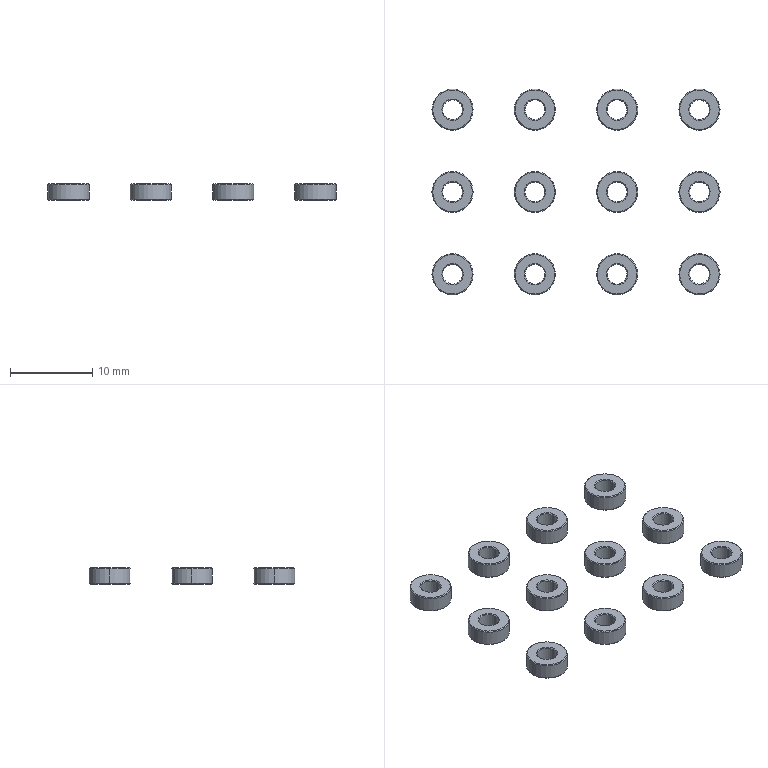NC program | NX | posted with a generic post | part box 35 x 25 x 2 mm
Lines 48 to 911 of 5177:
(ZLEVEL_PROFILE , TOOL : D4)
N88 T04 M6
N90 G54
N92 G17 G0 G90 X0.328 Y-1.531 S9500 M3
N94 G43 Z30. H4
N96 Z1.5
N98 G94 G1 X-0.348 Y-1.151 Z1.459 F1000.
N100 X-1.299 Y-0.146 Z1.387
N102 X-1.799 Y0.78 Z1.332
N104 X-2.099 Y1.969 Z1.267
N106 X-2.1 Y2.5 Z1.24
N108 Y3.026 Z1.212
N110 X-1.743 Y4.354 Z1.14
N112 X-1.012 Y5.517 Z1.068
N114 X0.029 Y6.415 Z0.996
N116 X1.287 Y6.968 Z0.924
N118 X2.653 Y7.127 Z0.852
N120 X4.005 Y6.879 Z0.78
N122 X4.954 Y6.426 Z0.725
N124 X6.004 Y5.526 Z0.652
N126 X6.742 Y4.356 Z0.58
N128 X7.101 Y3.021 Z0.507
N130 X7.099 Y1.969 Z0.452
N132 X6.909 Y1.087 Z0.405
N134 X6.551 Y0.258 Z0.358
N136 X5.94 Y-0.599 Z0.302
N138 X4.871 Y-1.477 Z0.23
N140 X3.59 Y-2. Z0.157
N142 X2.211 Y-2.121 Z0.085
N144 X0.858 Y-1.829 Z0.012
N146 X-0.348 Y-1.151 Z-0.06
N148 X-1.299 Y-0.146 Z-0.133
N150 X-1.799 Y0.78 Z-0.188
N152 X-2.099 Y1.969 Z-0.252
N154 X-2.1 Y2.5 Z-0.28
N156 G2 X2.5 Y7.1 R4.6 F2500.
N158 X-2.1 Y2.5 R-4.6
N160 G1 X-2.094 Y2.743 Z-0.284
N162 X-2.074 Y2.985 Z-0.288
N164 X-2.042 Y3.226 Z-0.293
N166 X-1.998 Y3.465 Z-0.297
N168 X-1.94 Y3.701 Z-0.301
N170 X-1.871 Y3.934 Z-0.305
N172 X-1.789 Y4.163 Z-0.31
N174 X-1.695 Y4.387 Z-0.314
N176 X-1.59 Y4.606 Z-0.318
N178 X-1.473 Y4.819 Z-0.322
N180 X-1.345 Y5.026 Z-0.327
N182 X-1.206 Y5.225 Z-0.331
N184 X-1.057 Y5.417 Z-0.335
N186 X-0.898 Y5.601 Z-0.339
N188 X-0.729 Y5.776 Z-0.344
N190 X-0.552 Y5.942 Z-0.348
N192 X-0.366 Y6.098 Z-0.352
N194 X-0.172 Y6.245 Z-0.356
N196 X0.03 Y6.38 Z-0.361
N198 X0.238 Y6.505 Z-0.365
N200 X0.453 Y6.619 Z-0.369
N202 X0.673 Y6.722 Z-0.373
N204 X0.899 Y6.812 Z-0.378
N206 X1.129 Y6.891 Z-0.382
N208 X1.362 Y6.957 Z-0.386
N210 X1.599 Y7.011 Z-0.39
N212 X1.839 Y7.052 Z-0.395
N214 X2.08 Y7.081 Z-0.399
N216 X2.323 Y7.097 Z-0.403
N218 X2.566 Y7.1 Z-0.407
N220 X2.809 Y7.09 Z-0.412
N222 X3.051 Y7.067 Z-0.416
N224 X3.291 Y7.031 Z-0.42
N226 X3.529 Y6.983 Z-0.424
N228 X3.765 Y6.923 Z-0.428
N230 X3.996 Y6.85 Z-0.433
N232 X4.224 Y6.765 Z-0.437
N234 X4.447 Y6.668 Z-0.441
N236 X4.664 Y6.559 Z-0.445
N238 X4.876 Y6.439 Z-0.45
N240 X5.08 Y6.308 Z-0.454
N242 X5.278 Y6.167 Z-0.458
N244 X5.468 Y6.015 Z-0.462
N246 X5.649 Y5.853 Z-0.467
N248 X5.822 Y5.682 Z-0.471
N250 X5.985 Y5.502 Z-0.475
N252 X6.139 Y5.314 Z-0.479
N254 X6.282 Y5.118 Z-0.484
N256 X6.415 Y4.915 Z-0.488
N258 X6.537 Y4.704 Z-0.492
N260 X6.648 Y4.488 Z-0.496
N262 X6.747 Y4.266 Z-0.501
N264 X6.835 Y4.039 Z-0.505
N266 X6.91 Y3.808 Z-0.509
N268 X6.973 Y3.574 Z-0.513
N270 X7.023 Y3.336 Z-0.518
N272 X7.061 Y3.096 Z-0.522
N274 X7.086 Y2.854 Z-0.526
N276 X7.099 Y2.611 Z-0.53
N278 X7.098 Y2.368 Z-0.535
N280 X7.085 Y2.126 Z-0.539
N282 X7.059 Y1.884 Z-0.543
N284 X7.02 Y1.644 Z-0.547
N286 X6.968 Y1.407 Z-0.552
N288 X6.904 Y1.172 Z-0.556
N290 X6.828 Y0.942 Z-0.56
N292 G2 X-2.1 Y2.5 R4.6
N294 G1 X-2.094 Y2.743 Z-0.564
N296 X-2.074 Y2.985 Z-0.568
N298 X-2.042 Y3.226 Z-0.573
N300 X-1.998 Y3.465 Z-0.577
N302 X-1.94 Y3.701 Z-0.581
N304 X-1.871 Y3.934 Z-0.585
N306 X-1.789 Y4.163 Z-0.59
N308 X-1.695 Y4.387 Z-0.594
N310 X-1.59 Y4.606 Z-0.598
N312 X-1.473 Y4.819 Z-0.602
N314 X-1.345 Y5.026 Z-0.607
N316 X-1.206 Y5.225 Z-0.611
N318 X-1.057 Y5.417 Z-0.615
N320 X-0.898 Y5.601 Z-0.619
N322 X-0.729 Y5.776 Z-0.624
N324 X-0.552 Y5.942 Z-0.628
N326 X-0.366 Y6.098 Z-0.632
N328 X-0.172 Y6.245 Z-0.636
N330 X0.03 Y6.38 Z-0.641
N332 X0.238 Y6.505 Z-0.645
N334 X0.453 Y6.619 Z-0.649
N336 X0.673 Y6.722 Z-0.653
N338 X0.899 Y6.812 Z-0.658
N340 X1.129 Y6.891 Z-0.662
N342 X1.362 Y6.957 Z-0.666
N344 X1.599 Y7.011 Z-0.67
N346 X1.839 Y7.052 Z-0.675
N348 X2.08 Y7.081 Z-0.679
N350 X2.323 Y7.097 Z-0.683
N352 X2.566 Y7.1 Z-0.687
N354 X2.809 Y7.09 Z-0.692
N356 X3.051 Y7.067 Z-0.696
N358 X3.291 Y7.031 Z-0.7
N360 X3.529 Y6.983 Z-0.704
N362 X3.765 Y6.923 Z-0.708
N364 X3.996 Y6.85 Z-0.713
N366 X4.224 Y6.765 Z-0.717
N368 X4.447 Y6.668 Z-0.721
N370 X4.664 Y6.559 Z-0.725
N372 X4.876 Y6.439 Z-0.73
N374 X5.08 Y6.308 Z-0.734
N376 X5.278 Y6.167 Z-0.738
N378 X5.468 Y6.015 Z-0.742
N380 X5.649 Y5.853 Z-0.747
N382 X5.822 Y5.682 Z-0.751
N384 X5.985 Y5.502 Z-0.755
N386 X6.139 Y5.314 Z-0.759
N388 X6.282 Y5.118 Z-0.764
N390 X6.415 Y4.915 Z-0.768
N392 X6.537 Y4.704 Z-0.772
N394 X6.648 Y4.488 Z-0.776
N396 X6.747 Y4.266 Z-0.781
N398 X6.835 Y4.039 Z-0.785
N400 X6.91 Y3.808 Z-0.789
N402 X6.973 Y3.574 Z-0.793
N404 X7.023 Y3.336 Z-0.798
N406 X7.061 Y3.096 Z-0.802
N408 X7.086 Y2.854 Z-0.806
N410 X7.099 Y2.611 Z-0.81
N412 X7.098 Y2.368 Z-0.815
N414 X7.085 Y2.126 Z-0.819
N416 X7.059 Y1.884 Z-0.823
N418 X7.02 Y1.644 Z-0.827
N420 X6.968 Y1.407 Z-0.832
N422 X6.904 Y1.172 Z-0.836
N424 X6.828 Y0.942 Z-0.84
N426 G2 X-2.1 Y2.5 R4.6
N428 G1 X-2.094 Y2.743 Z-0.844
N430 X-2.074 Y2.985 Z-0.848
N432 X-2.042 Y3.226 Z-0.853
N434 X-1.998 Y3.465 Z-0.857
N436 X-1.94 Y3.701 Z-0.861
N438 X-1.871 Y3.934 Z-0.865
N440 X-1.789 Y4.163 Z-0.87
N442 X-1.695 Y4.387 Z-0.874
N444 X-1.59 Y4.606 Z-0.878
N446 X-1.473 Y4.819 Z-0.882
N448 X-1.345 Y5.026 Z-0.887
N450 X-1.206 Y5.225 Z-0.891
N452 X-1.057 Y5.417 Z-0.895
N454 X-0.898 Y5.601 Z-0.899
N456 X-0.729 Y5.776 Z-0.904
N458 X-0.552 Y5.942 Z-0.908
N460 X-0.366 Y6.098 Z-0.912
N462 X-0.172 Y6.245 Z-0.916
N464 X0.03 Y6.38 Z-0.921
N466 X0.238 Y6.505 Z-0.925
N468 X0.453 Y6.619 Z-0.929
N470 X0.673 Y6.722 Z-0.933
N472 X0.899 Y6.812 Z-0.938
N474 X1.129 Y6.891 Z-0.942
N476 X1.362 Y6.957 Z-0.946
N478 X1.599 Y7.011 Z-0.95
N480 X1.839 Y7.052 Z-0.955
N482 X2.08 Y7.081 Z-0.959
N484 X2.323 Y7.097 Z-0.963
N486 X2.566 Y7.1 Z-0.967
N488 X2.809 Y7.09 Z-0.972
N490 X3.051 Y7.067 Z-0.976
N492 X3.291 Y7.031 Z-0.98
N494 X3.529 Y6.983 Z-0.984
N496 X3.765 Y6.923 Z-0.988
N498 X3.996 Y6.85 Z-0.993
N500 X4.224 Y6.765 Z-0.997
N502 X4.447 Y6.668 Z-1.001
N504 X4.664 Y6.559 Z-1.005
N506 X4.876 Y6.439 Z-1.01
N508 X5.08 Y6.308 Z-1.014
N510 X5.278 Y6.167 Z-1.018
N512 X5.468 Y6.015 Z-1.022
N514 X5.649 Y5.853 Z-1.027
N516 X5.822 Y5.682 Z-1.031
N518 X5.985 Y5.502 Z-1.035
N520 X6.139 Y5.314 Z-1.039
N522 X6.282 Y5.118 Z-1.044
N524 X6.415 Y4.915 Z-1.048
N526 X6.537 Y4.704 Z-1.052
N528 X6.648 Y4.488 Z-1.056
N530 X6.747 Y4.266 Z-1.061
N532 X6.835 Y4.039 Z-1.065
N534 X6.91 Y3.808 Z-1.069
N536 X6.973 Y3.574 Z-1.073
N538 X7.023 Y3.336 Z-1.078
N540 X7.061 Y3.096 Z-1.082
N542 X7.086 Y2.854 Z-1.086
N544 X7.099 Y2.611 Z-1.09
N546 X7.098 Y2.368 Z-1.095
N548 X7.085 Y2.126 Z-1.099
N550 X7.059 Y1.884 Z-1.103
N552 X7.02 Y1.644 Z-1.107
N554 X6.968 Y1.407 Z-1.112
N556 X6.904 Y1.172 Z-1.116
N558 X6.828 Y0.942 Z-1.12
N560 G2 X-2.1 Y2.5 R4.6
N562 G1 X-2.094 Y2.743 Z-1.124
N564 X-2.074 Y2.985 Z-1.128
N566 X-2.042 Y3.226 Z-1.133
N568 X-1.998 Y3.465 Z-1.137
N570 X-1.94 Y3.701 Z-1.141
N572 X-1.871 Y3.934 Z-1.145
N574 X-1.789 Y4.163 Z-1.15
N576 X-1.695 Y4.387 Z-1.154
N578 X-1.59 Y4.606 Z-1.158
N580 X-1.473 Y4.819 Z-1.162
N582 X-1.345 Y5.026 Z-1.167
N584 X-1.206 Y5.225 Z-1.171
N586 X-1.057 Y5.417 Z-1.175
N588 X-0.898 Y5.601 Z-1.179
N590 X-0.729 Y5.776 Z-1.184
N592 X-0.552 Y5.942 Z-1.188
N594 X-0.366 Y6.098 Z-1.192
N596 X-0.172 Y6.245 Z-1.196
N598 X0.03 Y6.38 Z-1.201
N600 X0.238 Y6.505 Z-1.205
N602 X0.453 Y6.619 Z-1.209
N604 X0.673 Y6.722 Z-1.213
N606 X0.899 Y6.812 Z-1.218
N608 X1.129 Y6.891 Z-1.222
N610 X1.362 Y6.957 Z-1.226
N612 X1.599 Y7.011 Z-1.23
N614 X1.839 Y7.052 Z-1.235
N616 X2.08 Y7.081 Z-1.239
N618 X2.323 Y7.097 Z-1.243
N620 X2.566 Y7.1 Z-1.247
N622 X2.809 Y7.09 Z-1.252
N624 X3.051 Y7.067 Z-1.256
N626 X3.291 Y7.031 Z-1.26
N628 X3.529 Y6.983 Z-1.264
N630 X3.765 Y6.923 Z-1.268
N632 X3.996 Y6.85 Z-1.273
N634 X4.224 Y6.765 Z-1.277
N636 X4.447 Y6.668 Z-1.281
N638 X4.664 Y6.559 Z-1.285
N640 X4.876 Y6.439 Z-1.29
N642 X5.08 Y6.308 Z-1.294
N644 X5.278 Y6.167 Z-1.298
N646 X5.468 Y6.015 Z-1.302
N648 X5.649 Y5.853 Z-1.307
N650 X5.822 Y5.682 Z-1.311
N652 X5.985 Y5.502 Z-1.315
N654 X6.139 Y5.314 Z-1.319
N656 X6.282 Y5.118 Z-1.324
N658 X6.415 Y4.915 Z-1.328
N660 X6.537 Y4.704 Z-1.332
N662 X6.648 Y4.488 Z-1.336
N664 X6.747 Y4.266 Z-1.341
N666 X6.835 Y4.039 Z-1.345
N668 X6.91 Y3.808 Z-1.349
N670 X6.973 Y3.574 Z-1.353
N672 X7.023 Y3.336 Z-1.358
N674 X7.061 Y3.096 Z-1.362
N676 X7.086 Y2.854 Z-1.366
N678 X7.099 Y2.611 Z-1.37
N680 X7.098 Y2.368 Z-1.375
N682 X7.085 Y2.126 Z-1.379
N684 X7.059 Y1.884 Z-1.383
N686 X7.02 Y1.644 Z-1.387
N688 X6.968 Y1.407 Z-1.392
N690 X6.904 Y1.172 Z-1.396
N692 X6.828 Y0.942 Z-1.4
N694 G2 X0.942 Y-1.828 R4.6
N696 X6.828 Y0.942 R-4.6
N698 G1 Z0.1
N700 G0 Z53.
N702 X16.567 Y0.295
N704 Z1.5
N706 G1 X16.551 Y0.258 Z1.498 F1000.
N708 X15.94 Y-0.599 Z1.443
N710 X15.1 Y-1.331 Z1.384
N712 X14.11 Y-1.841 Z1.326
N714 X13.026 Y-2.1 Z1.268
N716 X11.974 Z1.212
N718 X10.711 Y-1.77 Z1.144
N720 X9.59 Y-1.101 Z1.076
N722 X8.701 Y-0.146 Z1.007
N724 X8.201 Y0.78 Z0.952
N726 X7.901 Y1.969 Z0.888
N728 X7.899 Y3.021 Z0.833
N730 X8.256 Y4.35 Z0.761
N732 X8.986 Y5.515 Z0.689
N734 X10.027 Y6.414 Z0.616
N736 X11.286 Y6.968 Z0.544
N738 X12.652 Y7.128 Z0.472
N740 X14.005 Y6.879 Z0.4
N742 X14.954 Y6.426 Z0.345
N744 X16.004 Y5.526 Z0.273
N746 X16.742 Y4.356 Z0.2
N748 X17.101 Y3.021 Z0.128
N750 X17.099 Y1.969 Z0.072
N752 X16.909 Y1.087 Z0.025
N754 X16.551 Y0.258 Z-0.022
N756 X15.94 Y-0.599 Z-0.077
N758 X15.1 Y-1.331 Z-0.136
N760 X14.11 Y-1.841 Z-0.194
N762 X13.026 Y-2.1 Z-0.252
N764 X12.5 Z-0.28
N766 G2 X7.9 Y2.5 R4.6 F2500.
N768 X12.5 Y-2.1 R-4.6
N770 G1 X12.257 Y-2.094 Z-0.284
N772 X12.015 Y-2.074 Z-0.288
N774 X11.774 Y-2.042 Z-0.293
N776 X11.535 Y-1.998 Z-0.297
N778 X11.299 Y-1.94 Z-0.301
N780 X11.066 Y-1.871 Z-0.305
N782 X10.837 Y-1.789 Z-0.31
N784 X10.613 Y-1.695 Z-0.314
N786 X10.394 Y-1.59 Z-0.318
N788 X10.181 Y-1.473 Z-0.322
N790 X9.974 Y-1.345 Z-0.327
N792 X9.775 Y-1.206 Z-0.331
N794 X9.583 Y-1.057 Z-0.335
N796 X9.399 Y-0.898 Z-0.339
N798 X9.224 Y-0.729 Z-0.344
N800 X9.058 Y-0.552 Z-0.348
N802 X8.902 Y-0.366 Z-0.352
N804 X8.755 Y-0.172 Z-0.356
N806 X8.62 Y0.03 Z-0.361
N808 X8.495 Y0.238 Z-0.365
N810 X8.381 Y0.453 Z-0.369
N812 X8.278 Y0.673 Z-0.373
N814 X8.188 Y0.899 Z-0.378
N816 X8.109 Y1.129 Z-0.382
N818 X8.043 Y1.362 Z-0.386
N820 X7.989 Y1.599 Z-0.39
N822 X7.948 Y1.839 Z-0.395
N824 X7.919 Y2.08 Z-0.399
N826 X7.903 Y2.323 Z-0.403
N828 X7.9 Y2.566 Z-0.407
N830 X7.91 Y2.809 Z-0.412
N832 X7.933 Y3.051 Z-0.416
N834 X7.969 Y3.291 Z-0.42
N836 X8.017 Y3.529 Z-0.424
N838 X8.077 Y3.765 Z-0.428
N840 X8.15 Y3.996 Z-0.433
N842 X8.235 Y4.224 Z-0.437
N844 X8.332 Y4.447 Z-0.441
N846 X8.441 Y4.664 Z-0.445
N848 X8.561 Y4.876 Z-0.45
N850 X8.692 Y5.08 Z-0.454
N852 X8.833 Y5.278 Z-0.458
N854 X8.985 Y5.468 Z-0.462
N856 X9.147 Y5.649 Z-0.467
N858 X9.318 Y5.822 Z-0.471
N860 X9.498 Y5.985 Z-0.475
N862 X9.686 Y6.139 Z-0.479
N864 X9.882 Y6.282 Z-0.484
N866 X10.085 Y6.415 Z-0.488
N868 X10.296 Y6.537 Z-0.492
N870 X10.512 Y6.648 Z-0.496
N872 X10.734 Y6.747 Z-0.501
N874 X10.961 Y6.835 Z-0.505
N876 X11.192 Y6.91 Z-0.509
N878 X11.426 Y6.973 Z-0.513
N880 X11.664 Y7.023 Z-0.518
N882 X11.904 Y7.061 Z-0.522
N884 X12.146 Y7.086 Z-0.526
N886 X12.389 Y7.099 Z-0.53
N888 X12.632 Y7.098 Z-0.535
N890 X12.874 Y7.085 Z-0.539
N892 X13.116 Y7.059 Z-0.543
N894 X13.356 Y7.02 Z-0.547
N896 X13.593 Y6.968 Z-0.552
N898 X13.828 Y6.904 Z-0.556
N900 X14.058 Y6.828 Z-0.56
N902 G2 X12.5 Y-2.1 R4.6
N904 G1 X12.257 Y-2.094 Z-0.564
N906 X12.015 Y-2.074 Z-0.568
N908 X11.774 Y-2.042 Z-0.573
N910 X11.535 Y-1.998 Z-0.577
N912 X11.299 Y-1.94 Z-0.581
N914 X11.066 Y-1.871 Z-0.585
N916 X10.837 Y-1.789 Z-0.59
N918 X10.613 Y-1.695 Z-0.594
N920 X10.394 Y-1.59 Z-0.598
N922 X10.181 Y-1.473 Z-0.602
N924 X9.974 Y-1.345 Z-0.607
N926 X9.775 Y-1.206 Z-0.611
N928 X9.583 Y-1.057 Z-0.615
N930 X9.399 Y-0.898 Z-0.619
N932 X9.224 Y-0.729 Z-0.624
N934 X9.058 Y-0.552 Z-0.628
N936 X8.902 Y-0.366 Z-0.632
N938 X8.755 Y-0.172 Z-0.636
N940 X8.62 Y0.03 Z-0.641
N942 X8.495 Y0.238 Z-0.645
N944 X8.381 Y0.453 Z-0.649
N946 X8.278 Y0.673 Z-0.653
N948 X8.188 Y0.899 Z-0.658
N950 X8.109 Y1.129 Z-0.662
N952 X8.043 Y1.362 Z-0.666
N954 X7.989 Y1.599 Z-0.67
N956 X7.948 Y1.839 Z-0.675
N958 X7.919 Y2.08 Z-0.679
N960 X7.903 Y2.323 Z-0.683
N962 X7.9 Y2.566 Z-0.687
N964 X7.91 Y2.809 Z-0.692
N966 X7.933 Y3.051 Z-0.696
N968 X7.969 Y3.291 Z-0.7
N970 X8.017 Y3.529 Z-0.704
N972 X8.077 Y3.765 Z-0.708
N974 X8.15 Y3.996 Z-0.713
N976 X8.235 Y4.224 Z-0.717
N978 X8.332 Y4.447 Z-0.721
N980 X8.441 Y4.664 Z-0.725
N982 X8.561 Y4.876 Z-0.73
N984 X8.692 Y5.08 Z-0.734
N986 X8.833 Y5.278 Z-0.738
N988 X8.985 Y5.468 Z-0.742
N990 X9.147 Y5.649 Z-0.747
N992 X9.318 Y5.822 Z-0.751
N994 X9.498 Y5.985 Z-0.755
N996 X9.686 Y6.139 Z-0.759
N998 X9.882 Y6.282 Z-0.764
N1000 X10.085 Y6.415 Z-0.768
N1002 X10.296 Y6.537 Z-0.772
N1004 X10.512 Y6.648 Z-0.776
N1006 X10.734 Y6.747 Z-0.781
N1008 X10.961 Y6.835 Z-0.785
N1010 X11.192 Y6.91 Z-0.789
N1012 X11.426 Y6.973 Z-0.793
N1014 X11.664 Y7.023 Z-0.798
N1016 X11.904 Y7.061 Z-0.802
N1018 X12.146 Y7.086 Z-0.806
N1020 X12.389 Y7.099 Z-0.81
N1022 X12.632 Y7.098 Z-0.815
N1024 X12.874 Y7.085 Z-0.819
N1026 X13.116 Y7.059 Z-0.823
N1028 X13.356 Y7.02 Z-0.827
N1030 X13.593 Y6.968 Z-0.832
N1032 X13.828 Y6.904 Z-0.836
N1034 X14.058 Y6.828 Z-0.84
N1036 G2 X12.5 Y-2.1 R4.6
N1038 G1 X12.257 Y-2.094 Z-0.844
N1040 X12.015 Y-2.074 Z-0.848
N1042 X11.774 Y-2.042 Z-0.853
N1044 X11.535 Y-1.998 Z-0.857
N1046 X11.299 Y-1.94 Z-0.861
N1048 X11.066 Y-1.871 Z-0.865
N1050 X10.837 Y-1.789 Z-0.87
N1052 X10.613 Y-1.695 Z-0.874
N1054 X10.394 Y-1.59 Z-0.878
N1056 X10.181 Y-1.473 Z-0.882
N1058 X9.974 Y-1.345 Z-0.887
N1060 X9.775 Y-1.206 Z-0.891
N1062 X9.583 Y-1.057 Z-0.895
N1064 X9.399 Y-0.898 Z-0.899
N1066 X9.224 Y-0.729 Z-0.904
N1068 X9.058 Y-0.552 Z-0.908
N1070 X8.902 Y-0.366 Z-0.912
N1072 X8.755 Y-0.172 Z-0.916
N1074 X8.62 Y0.03 Z-0.921
N1076 X8.495 Y0.238 Z-0.925
N1078 X8.381 Y0.453 Z-0.929
N1080 X8.278 Y0.673 Z-0.933
N1082 X8.188 Y0.899 Z-0.938
N1084 X8.109 Y1.129 Z-0.942
N1086 X8.043 Y1.362 Z-0.946
N1088 X7.989 Y1.599 Z-0.95
N1090 X7.948 Y1.839 Z-0.955
N1092 X7.919 Y2.08 Z-0.959
N1094 X7.903 Y2.323 Z-0.963
N1096 X7.9 Y2.566 Z-0.967
N1098 X7.91 Y2.809 Z-0.972
N1100 X7.933 Y3.051 Z-0.976
N1102 X7.969 Y3.291 Z-0.98
N1104 X8.017 Y3.529 Z-0.984
N1106 X8.077 Y3.765 Z-0.988
N1108 X8.15 Y3.996 Z-0.993
N1110 X8.235 Y4.224 Z-0.997
N1112 X8.332 Y4.447 Z-1.001
N1114 X8.441 Y4.664 Z-1.005
N1116 X8.561 Y4.876 Z-1.01
N1118 X8.692 Y5.08 Z-1.014
N1120 X8.833 Y5.278 Z-1.018
N1122 X8.985 Y5.468 Z-1.022
N1124 X9.147 Y5.649 Z-1.027
N1126 X9.318 Y5.822 Z-1.031
N1128 X9.498 Y5.985 Z-1.035
N1130 X9.686 Y6.139 Z-1.039
N1132 X9.882 Y6.282 Z-1.044
N1134 X10.085 Y6.415 Z-1.048
N1136 X10.296 Y6.537 Z-1.052
N1138 X10.512 Y6.648 Z-1.056
N1140 X10.734 Y6.747 Z-1.061
N1142 X10.961 Y6.835 Z-1.065
N1144 X11.192 Y6.91 Z-1.069
N1146 X11.426 Y6.973 Z-1.073
N1148 X11.664 Y7.023 Z-1.078
N1150 X11.904 Y7.061 Z-1.082
N1152 X12.146 Y7.086 Z-1.086
N1154 X12.389 Y7.099 Z-1.09
N1156 X12.632 Y7.098 Z-1.095
N1158 X12.874 Y7.085 Z-1.099
N1160 X13.116 Y7.059 Z-1.103
N1162 X13.356 Y7.02 Z-1.107
N1164 X13.593 Y6.968 Z-1.112
N1166 X13.828 Y6.904 Z-1.116
N1168 X14.058 Y6.828 Z-1.12
N1170 G2 X12.5 Y-2.1 R4.6
N1172 G1 X12.257 Y-2.094 Z-1.124
N1174 X12.015 Y-2.074 Z-1.128
N1176 X11.774 Y-2.042 Z-1.133
N1178 X11.535 Y-1.998 Z-1.137
N1180 X11.299 Y-1.94 Z-1.141
N1182 X11.066 Y-1.871 Z-1.145
N1184 X10.837 Y-1.789 Z-1.15
N1186 X10.613 Y-1.695 Z-1.154
N1188 X10.394 Y-1.59 Z-1.158
N1190 X10.181 Y-1.473 Z-1.162
N1192 X9.974 Y-1.345 Z-1.167
N1194 X9.775 Y-1.206 Z-1.171
N1196 X9.583 Y-1.057 Z-1.175
N1198 X9.399 Y-0.898 Z-1.179
N1200 X9.224 Y-0.729 Z-1.184
N1202 X9.058 Y-0.552 Z-1.188
N1204 X8.902 Y-0.366 Z-1.192
N1206 X8.755 Y-0.172 Z-1.196
N1208 X8.62 Y0.03 Z-1.201
N1210 X8.495 Y0.238 Z-1.205
N1212 X8.381 Y0.453 Z-1.209
N1214 X8.278 Y0.673 Z-1.213
N1216 X8.188 Y0.899 Z-1.218
N1218 X8.109 Y1.129 Z-1.222
N1220 X8.043 Y1.362 Z-1.226
N1222 X7.989 Y1.599 Z-1.23
N1224 X7.948 Y1.839 Z-1.235
N1226 X7.919 Y2.08 Z-1.239
N1228 X7.903 Y2.323 Z-1.243
N1230 X7.9 Y2.566 Z-1.247
N1232 X7.91 Y2.809 Z-1.252
N1234 X7.933 Y3.051 Z-1.256
N1236 X7.969 Y3.291 Z-1.26
N1238 X8.017 Y3.529 Z-1.264
N1240 X8.077 Y3.765 Z-1.268
N1242 X8.15 Y3.996 Z-1.273
N1244 X8.235 Y4.224 Z-1.277
N1246 X8.332 Y4.447 Z-1.281
N1248 X8.441 Y4.664 Z-1.285
N1250 X8.561 Y4.876 Z-1.29
N1252 X8.692 Y5.08 Z-1.294
N1254 X8.833 Y5.278 Z-1.298
N1256 X8.985 Y5.468 Z-1.302
N1258 X9.147 Y5.649 Z-1.307
N1260 X9.318 Y5.822 Z-1.311
N1262 X9.498 Y5.985 Z-1.315
N1264 X9.686 Y6.139 Z-1.319
N1266 X9.882 Y6.282 Z-1.324
N1268 X10.085 Y6.415 Z-1.328
N1270 X10.296 Y6.537 Z-1.332
N1272 X10.512 Y6.648 Z-1.336
N1274 X10.734 Y6.747 Z-1.341
N1276 X10.961 Y6.835 Z-1.345
N1278 X11.192 Y6.91 Z-1.349
N1280 X11.426 Y6.973 Z-1.353
N1282 X11.664 Y7.023 Z-1.358
N1284 X11.904 Y7.061 Z-1.362
N1286 X12.146 Y7.086 Z-1.366
N1288 X12.389 Y7.099 Z-1.37
N1290 X12.632 Y7.098 Z-1.375
N1292 X12.874 Y7.085 Z-1.379
N1294 X13.116 Y7.059 Z-1.383
N1296 X13.356 Y7.02 Z-1.387
N1298 X13.593 Y6.968 Z-1.392
N1300 X13.828 Y6.904 Z-1.396
N1302 X14.058 Y6.828 Z-1.4
N1304 G2 X16.828 Y0.942 R4.6
N1306 X14.058 Y6.828 R-4.6
N1308 G1 Z0.1
N1310 G0 Z53.
N1312 X8.464 Y24.685
N1314 Z1.5
N1316 G1 X8.819 Y25.308 Z1.462 F1000.
N1318 X9.696 Y26.184 Z1.397
N1320 X10.773 Y26.796 Z1.333
N1322 X11.974 Y27.1 Z1.268
N1324 X13.026 Z1.212
N1326 X14.049 Y26.863 Z1.157
N1328 X14.994 Y26.401 Z1.102
N1330 X16.023 Y25.505 Z1.031
N1332 X16.745 Y24.348 Z0.959
N1334 X17.099 Y23.031 Z0.888
N1336 X17.101 Y21.979 Z0.833
N1338 X16.907 Y21.08 Z0.785
N1340 X16.539 Y20.236 Z0.736
N1342 X15.923 Y19.383 Z0.681
N1344 X14.856 Y18.514 Z0.609
N1346 X13.581 Y17.998 Z0.537
N1348 X12.21 Y17.879 Z0.465
N1350 X10.865 Y18.168 Z0.393
N1352 X9.664 Y18.84 Z0.321
N1354 X8.714 Y19.835 Z0.248
N1356 X8.21 Y20.759 Z0.193
N1358 X7.899 Y21.979 Z0.127
N1360 X7.901 Y23.031 Z0.072
N1362 X8.206 Y24.232 Z0.007
N1364 X8.819 Y25.308 Z-0.058
N1366 X9.696 Y26.184 Z-0.123
N1368 X10.773 Y26.796 Z-0.187
N1370 X11.974 Y27.1 Z-0.252
N1372 X12.5 Z-0.28
N1374 G2 X17.1 Y22.5 R4.6 F2500.
N1376 X12.5 Y27.1 R-4.6
N1378 G1 X12.743 Y27.094 Z-0.284
N1380 X12.985 Y27.074 Z-0.288
N1382 X13.226 Y27.042 Z-0.293
N1384 X13.465 Y26.998 Z-0.297
N1386 X13.701 Y26.94 Z-0.301
N1388 X13.934 Y26.871 Z-0.305
N1390 X14.163 Y26.789 Z-0.31
N1392 X14.387 Y26.695 Z-0.314
N1394 X14.606 Y26.59 Z-0.318
N1396 X14.819 Y26.473 Z-0.322
N1398 X15.026 Y26.345 Z-0.327
N1400 X15.225 Y26.206 Z-0.331
N1402 X15.417 Y26.057 Z-0.335
N1404 X15.601 Y25.898 Z-0.339
N1406 X15.776 Y25.729 Z-0.344
N1408 X15.942 Y25.552 Z-0.348
N1410 X16.098 Y25.366 Z-0.352
N1412 X16.245 Y25.172 Z-0.356
N1414 X16.38 Y24.97 Z-0.361
N1416 X16.505 Y24.762 Z-0.365
N1418 X16.619 Y24.547 Z-0.369
N1420 X16.722 Y24.327 Z-0.373
N1422 X16.812 Y24.101 Z-0.378
N1424 X16.891 Y23.871 Z-0.382
N1426 X16.957 Y23.638 Z-0.386
N1428 X17.011 Y23.401 Z-0.39
N1430 X17.052 Y23.161 Z-0.395
N1432 X17.081 Y22.92 Z-0.399
N1434 X17.097 Y22.677 Z-0.403
N1436 X17.1 Y22.434 Z-0.407
N1438 X17.09 Y22.191 Z-0.412
N1440 X17.067 Y21.949 Z-0.416
N1442 X17.031 Y21.709 Z-0.42
N1444 X16.983 Y21.471 Z-0.424
N1446 X16.923 Y21.235 Z-0.428
N1448 X16.85 Y21.004 Z-0.433
N1450 X16.765 Y20.776 Z-0.437
N1452 X16.668 Y20.553 Z-0.441
N1454 X16.559 Y20.336 Z-0.445
N1456 X16.439 Y20.124 Z-0.45
N1458 X16.308 Y19.92 Z-0.454
N1460 X16.167 Y19.722 Z-0.458
N1462 X16.015 Y19.532 Z-0.462
N1464 X15.853 Y19.351 Z-0.467
N1466 X15.682 Y19.178 Z-0.471
N1468 X15.502 Y19.015 Z-0.475
N1470 X15.314 Y18.861 Z-0.479
N1472 X15.118 Y18.718 Z-0.484
N1474 X14.915 Y18.585 Z-0.488
N1476 X14.704 Y18.463 Z-0.492
N1478 X14.488 Y18.352 Z-0.496
N1480 X14.266 Y18.253 Z-0.501
N1482 X14.039 Y18.165 Z-0.505
N1484 X13.808 Y18.09 Z-0.509
N1486 X13.574 Y18.027 Z-0.513
N1488 X13.336 Y17.977 Z-0.518
N1490 X13.096 Y17.939 Z-0.522
N1492 X12.854 Y17.914 Z-0.526
N1494 X12.611 Y17.901 Z-0.53
N1496 X12.368 Y17.902 Z-0.535
N1498 X12.126 Y17.915 Z-0.539
N1500 X11.884 Y17.941 Z-0.543
N1502 X11.644 Y17.98 Z-0.547
N1504 X11.407 Y18.032 Z-0.552
N1506 X11.172 Y18.096 Z-0.556
N1508 X10.942 Y18.172 Z-0.56
N1510 G2 X12.5 Y27.1 R4.6
N1512 G1 X12.743 Y27.094 Z-0.564
N1514 X12.985 Y27.074 Z-0.568
N1516 X13.226 Y27.042 Z-0.573
N1518 X13.465 Y26.998 Z-0.577
N1520 X13.701 Y26.94 Z-0.581
N1522 X13.934 Y26.871 Z-0.585
N1524 X14.163 Y26.789 Z-0.59
N1526 X14.387 Y26.695 Z-0.594
N1528 X14.606 Y26.59 Z-0.598
N1530 X14.819 Y26.473 Z-0.602
N1532 X15.026 Y26.345 Z-0.607
N1534 X15.225 Y26.206 Z-0.611
N1536 X15.417 Y26.057 Z-0.615
N1538 X15.601 Y25.898 Z-0.619
N1540 X15.776 Y25.729 Z-0.624
N1542 X15.942 Y25.552 Z-0.628
N1544 X16.098 Y25.366 Z-0.632
N1546 X16.245 Y25.172 Z-0.636
N1548 X16.38 Y24.97 Z-0.641
N1550 X16.505 Y24.762 Z-0.645
N1552 X16.619 Y24.547 Z-0.649
N1554 X16.722 Y24.327 Z-0.653
N1556 X16.812 Y24.101 Z-0.658
N1558 X16.891 Y23.871 Z-0.662
N1560 X16.957 Y23.638 Z-0.666
N1562 X17.011 Y23.401 Z-0.67
N1564 X17.052 Y23.161 Z-0.675
N1566 X17.081 Y22.92 Z-0.679
N1568 X17.097 Y22.677 Z-0.683
N1570 X17.1 Y22.434 Z-0.687
N1572 X17.09 Y22.191 Z-0.692
N1574 X17.067 Y21.949 Z-0.696
N1576 X17.031 Y21.709 Z-0.7
N1578 X16.983 Y21.471 Z-0.704
N1580 X16.923 Y21.235 Z-0.708
N1582 X16.85 Y21.004 Z-0.713
N1584 X16.765 Y20.776 Z-0.717
N1586 X16.668 Y20.553 Z-0.721
N1588 X16.559 Y20.336 Z-0.725
N1590 X16.439 Y20.124 Z-0.73
N1592 X16.308 Y19.92 Z-0.734
N1594 X16.167 Y19.722 Z-0.738
N1596 X16.015 Y19.532 Z-0.742
N1598 X15.853 Y19.351 Z-0.747
N1600 X15.682 Y19.178 Z-0.751
N1602 X15.502 Y19.015 Z-0.755
N1604 X15.314 Y18.861 Z-0.759
N1606 X15.118 Y18.718 Z-0.764
N1608 X14.915 Y18.585 Z-0.768
N1610 X14.704 Y18.463 Z-0.772
N1612 X14.488 Y18.352 Z-0.776
N1614 X14.266 Y18.253 Z-0.781
N1616 X14.039 Y18.165 Z-0.785
N1618 X13.808 Y18.09 Z-0.789
N1620 X13.574 Y18.027 Z-0.793
N1622 X13.336 Y17.977 Z-0.798
N1624 X13.096 Y17.939 Z-0.802
N1626 X12.854 Y17.914 Z-0.806
N1628 X12.611 Y17.901 Z-0.81
N1630 X12.368 Y17.902 Z-0.815
N1632 X12.126 Y17.915 Z-0.819
N1634 X11.884 Y17.941 Z-0.823
N1636 X11.644 Y17.98 Z-0.827
N1638 X11.407 Y18.032 Z-0.832
N1640 X11.172 Y18.096 Z-0.836
N1642 X10.942 Y18.172 Z-0.84
N1644 G2 X12.5 Y27.1 R4.6
N1646 G1 X12.743 Y27.094 Z-0.844
N1648 X12.985 Y27.074 Z-0.848
N1650 X13.226 Y27.042 Z-0.853
N1652 X13.465 Y26.998 Z-0.857
N1654 X13.701 Y26.94 Z-0.861
N1656 X13.934 Y26.871 Z-0.865
N1658 X14.163 Y26.789 Z-0.87
N1660 X14.387 Y26.695 Z-0.874
N1662 X14.606 Y26.59 Z-0.878
N1664 X14.819 Y26.473 Z-0.882
N1666 X15.026 Y26.345 Z-0.887
N1668 X15.225 Y26.206 Z-0.891
N1670 X15.417 Y26.057 Z-0.895
N1672 X15.601 Y25.898 Z-0.899
N1674 X15.776 Y25.729 Z-0.904
N1676 X15.942 Y25.552 Z-0.908
N1678 X16.098 Y25.366 Z-0.912
N1680 X16.245 Y25.172 Z-0.916
N1682 X16.38 Y24.97 Z-0.921
N1684 X16.505 Y24.762 Z-0.925
N1686 X16.619 Y24.547 Z-0.929
N1688 X16.722 Y24.327 Z-0.933
N1690 X16.812 Y24.101 Z-0.938
N1692 X16.891 Y23.871 Z-0.942
N1694 X16.957 Y23.638 Z-0.946
N1696 X17.011 Y23.401 Z-0.95
N1698 X17.052 Y23.161 Z-0.955
N1700 X17.081 Y22.92 Z-0.959
N1702 X17.097 Y22.677 Z-0.963
N1704 X17.1 Y22.434 Z-0.967
N1706 X17.09 Y22.191 Z-0.972
N1708 X17.067 Y21.949 Z-0.976
N1710 X17.031 Y21.709 Z-0.98
N1712 X16.983 Y21.471 Z-0.984
N1714 X16.923 Y21.235 Z-0.988
N1716 X16.85 Y21.004 Z-0.993
N1718 X16.765 Y20.776 Z-0.997
N1720 X16.668 Y20.553 Z-1.001
N1722 X16.559 Y20.336 Z-1.005
N1724 X16.439 Y20.124 Z-1.01
N1726 X16.308 Y19.92 Z-1.014
N1728 X16.167 Y19.722 Z-1.018
N1730 X16.015 Y19.532 Z-1.022
N1732 X15.853 Y19.351 Z-1.027
N1734 X15.682 Y19.178 Z-1.031
N1736 X15.502 Y19.015 Z-1.035
N1738 X15.314 Y18.861 Z-1.039
N1740 X15.118 Y18.718 Z-1.044
N1742 X14.915 Y18.585 Z-1.048
N1744 X14.704 Y18.463 Z-1.052
N1746 X14.488 Y18.352 Z-1.056
N1748 X14.266 Y18.253 Z-1.061
N1750 X14.039 Y18.165 Z-1.065
N1752 X13.808 Y18.09 Z-1.069
N1754 X13.574 Y18.027 Z-1.073
N1756 X13.336 Y17.977 Z-1.078
N1758 X13.096 Y17.939 Z-1.082
N1760 X12.854 Y17.914 Z-1.086
N1762 X12.611 Y17.901 Z-1.09
N1764 X12.368 Y17.902 Z-1.095
N1766 X12.126 Y17.915 Z-1.099
N1768 X11.884 Y17.941 Z-1.103
N1770 X11.644 Y17.98 Z-1.107
N1772 X11.407 Y18.032 Z-1.112
N1774 X11.172 Y18.096 Z-1.116
N1776 X10.942 Y18.172 Z-1.12
N1778 G2 X12.5 Y27.1 R4.6
N1780 G1 X12.743 Y27.094 Z-1.124
N1782 X12.985 Y27.074 Z-1.128
N1784 X13.226 Y27.042 Z-1.133
N1786 X13.465 Y26.998 Z-1.137
N1788 X13.701 Y26.94 Z-1.141
N1790 X13.934 Y26.871 Z-1.145
N1792 X14.163 Y26.789 Z-1.15
N1794 X14.387 Y26.695 Z-1.154
N1796 X14.606 Y26.59 Z-1.158
N1798 X14.819 Y26.473 Z-1.162
N1800 X15.026 Y26.345 Z-1.167
N1802 X15.225 Y26.206 Z-1.171
N1804 X15.417 Y26.057 Z-1.175
N1806 X15.601 Y25.898 Z-1.179
N1808 X15.776 Y25.729 Z-1.184